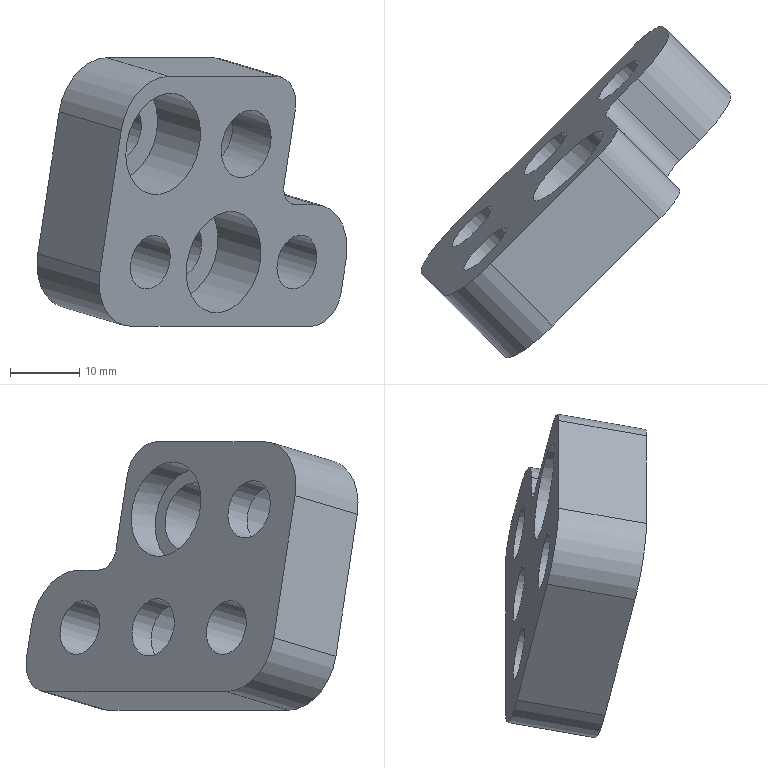Part | STEP file | gslz 2016.10.28-13_id90_x_t | 1 solid | 25 faces | box 44.883 x 48.072 x 38.894 mm | volume 13355 mm3 | cylinder 14 | plane 11 | commonest cylinder face diameters 10 x3 16 x3 8 x2 8.5 x2 15 x2 6 x1